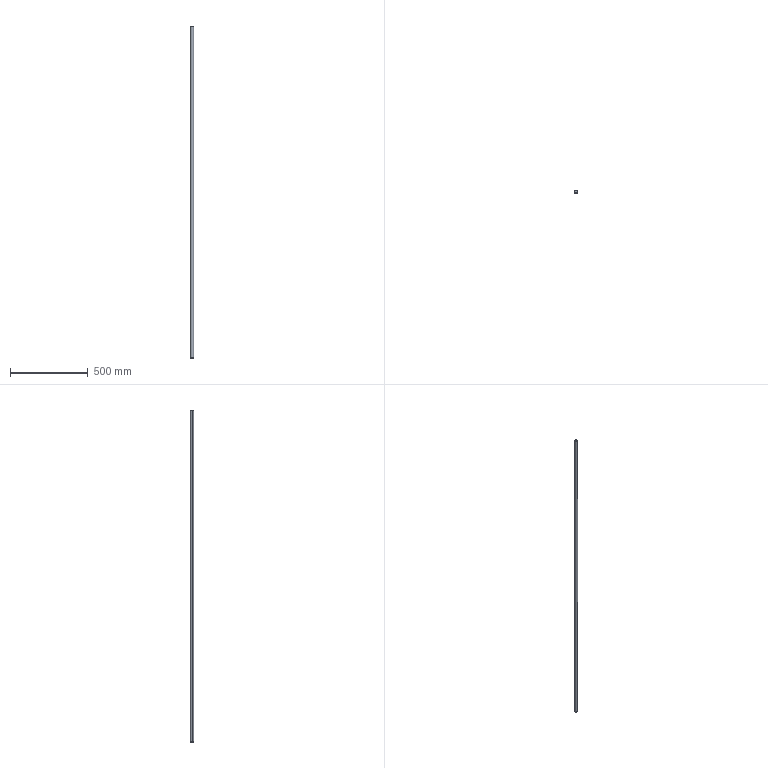Part | SolidWorks | features Chamfer 1, Extrusion 1 | 1 solid | 8 faces | box 20 x 20 x 2135 mm | volume 670495 mm3 | cone 4 | cylinder 2 | plane 2 | commonest cylinder face diameters 20 x2
STEP:
#1=CARTESIAN_POINT('',(8.,0.,2135.));
#2=VERTEX_POINT('',#1);
#3=CARTESIAN_POINT('',(-8.,0.,2135.));
#4=VERTEX_POINT('',#3);
#5=CARTESIAN_POINT('',(0.,0.,2135.));
#6=DIRECTION('',(0.,0.,1.));
#7=DIRECTION('',(1.,0.,0.));
#8=AXIS2_PLACEMENT_3D('',#5,#6,#7);
#9=CIRCLE('',#8,8.);
#10=EDGE_CURVE('',#2,#4,#9,.T.);
#11=ORIENTED_EDGE('',*,*,#10,.F.);
#12=CARTESIAN_POINT('',(10.,0.,2133.));
#13=VERTEX_POINT('',#12);
#14=CARTESIAN_POINT('',(8.,0.,2135.));
#15=DIRECTION('',(0.7071,0.,-0.7071));
#16=VECTOR('',#15,1000.);
#17=LINE('',#14,#16);
#18=EDGE_CURVE('',#2,#13,#17,.T.);
#19=ORIENTED_EDGE('',*,*,#18,.T.);
#20=CARTESIAN_POINT('',(-10.,0.,2133.));
#21=VERTEX_POINT('',#20);
#22=CARTESIAN_POINT('',(0.,0.,2133.));
#23=DIRECTION('',(0.,0.,-1.));
#24=DIRECTION('',(1.,0.,0.));
#25=AXIS2_PLACEMENT_3D('',#22,#23,#24);
#26=CIRCLE('',#25,10.);
#27=EDGE_CURVE('',#21,#13,#26,.T.);
#28=ORIENTED_EDGE('',*,*,#27,.F.);
#29=CARTESIAN_POINT('',(-8.,0.,2135.));
#30=DIRECTION('',(-0.7071,0.,-0.7071));
#31=VECTOR('',#30,1000.);
#32=LINE('',#29,#31);
#33=EDGE_CURVE('',#4,#21,#32,.T.);
#34=ORIENTED_EDGE('',*,*,#33,.F.);
#35=EDGE_LOOP('',(#11,#19,#28,#34));
#36=FACE_OUTER_BOUND('',#35,.T.);
#37=CARTESIAN_POINT('',(0.,0.,2135.));
#38=DIRECTION('',(0.,0.,-1.));
#39=DIRECTION('',(-1.,0.,0.));
#40=AXIS2_PLACEMENT_3D('',#37,#38,#39);
#41=CONICAL_SURFACE('',#40,8.,0.7854);
#42=ADVANCED_FACE('',(#36),#41,.T.);
#43=CARTESIAN_POINT('',(-8.,0.,0.));
#44=VERTEX_POINT('',#43);
#45=CARTESIAN_POINT('',(8.,0.,0.));
#46=VERTEX_POINT('',#45);
#47=CARTESIAN_POINT('',(0.,0.,0.));
#48=DIRECTION('',(0.,0.,-1.));
#49=DIRECTION('',(1.,0.,0.));
#50=AXIS2_PLACEMENT_3D('',#47,#48,#49);
#51=CIRCLE('',#50,8.);
#52=EDGE_CURVE('',#44,#46,#51,.T.);
#53=ORIENTED_EDGE('',*,*,#52,.F.);
#54=CARTESIAN_POINT('',(-10.,0.,2.));
#55=VERTEX_POINT('',#54);
#56=CARTESIAN_POINT('',(-10.,0.,2.));
#57=DIRECTION('',(-0.7071,0.,0.7071));
#58=VECTOR('',#57,1000.);
#59=LINE('',#56,#58);
#60=EDGE_CURVE('',#44,#55,#59,.T.);
#61=ORIENTED_EDGE('',*,*,#60,.T.);
#62=CARTESIAN_POINT('',(10.,0.,2.));
#63=VERTEX_POINT('',#62);
#64=CARTESIAN_POINT('',(0.,0.,2.));
#65=DIRECTION('',(0.,0.,1.));
#66=DIRECTION('',(1.,0.,0.));
#67=AXIS2_PLACEMENT_3D('',#64,#65,#66);
#68=CIRCLE('',#67,10.);
#69=EDGE_CURVE('',#63,#55,#68,.T.);
#70=ORIENTED_EDGE('',*,*,#69,.F.);
#71=CARTESIAN_POINT('',(10.,0.,2.));
#72=DIRECTION('',(0.7071,0.,0.7071));
#73=VECTOR('',#72,1000.);
#74=LINE('',#71,#73);
#75=EDGE_CURVE('',#46,#63,#74,.T.);
#76=ORIENTED_EDGE('',*,*,#75,.F.);
#77=EDGE_LOOP('',(#53,#61,#70,#76));
#78=FACE_OUTER_BOUND('',#77,.T.);
#79=CARTESIAN_POINT('',(0.,0.,2.));
#80=DIRECTION('',(0.,0.,1.));
#81=DIRECTION('',(1.,0.,0.));
#82=AXIS2_PLACEMENT_3D('',#79,#80,#81);
#83=CONICAL_SURFACE('',#82,10.,0.7854);
#84=ADVANCED_FACE('',(#78),#83,.T.);
#85=ORIENTED_EDGE('',*,*,#27,.T.);
#86=CARTESIAN_POINT('',(10.,0.,2135.));
#87=DIRECTION('',(0.,0.,-1.));
#88=VECTOR('',#87,1000.);
#89=LINE('',#86,#88);
#90=EDGE_CURVE('',#13,#63,#89,.T.);
#91=ORIENTED_EDGE('',*,*,#90,.T.);
#92=ORIENTED_EDGE('',*,*,#69,.T.);
#93=CARTESIAN_POINT('',(-10.,0.,2135.));
#94=DIRECTION('',(0.,0.,-1.));
#95=VECTOR('',#94,1000.);
#96=LINE('',#93,#95);
#97=EDGE_CURVE('',#21,#55,#96,.T.);
#98=ORIENTED_EDGE('',*,*,#97,.F.);
#99=EDGE_LOOP('',(#85,#91,#92,#98));
#100=FACE_OUTER_BOUND('',#99,.T.);
#101=CARTESIAN_POINT('',(0.,0.,2135.));
#102=DIRECTION('',(0.,0.,-1.));
#103=DIRECTION('',(-1.,0.,0.));
#104=AXIS2_PLACEMENT_3D('',#101,#102,#103);
#105=CYLINDRICAL_SURFACE('',#104,10.);
#106=ADVANCED_FACE('',(#100),#105,.T.);
#107=ORIENTED_EDGE('',*,*,#90,.F.);
#108=CARTESIAN_POINT('',(0.,0.,2133.));
#109=DIRECTION('',(0.,0.,-1.));
#110=DIRECTION('',(1.,0.,0.));
#111=AXIS2_PLACEMENT_3D('',#108,#109,#110);
#112=CIRCLE('',#111,10.);
#113=EDGE_CURVE('',#13,#21,#112,.T.);
#114=ORIENTED_EDGE('',*,*,#113,.T.);
#115=ORIENTED_EDGE('',*,*,#97,.T.);
#116=CARTESIAN_POINT('',(0.,0.,2.));
#117=DIRECTION('',(0.,0.,1.));
#118=DIRECTION('',(1.,0.,0.));
#119=AXIS2_PLACEMENT_3D('',#116,#117,#118);
#120=CIRCLE('',#119,10.);
#121=EDGE_CURVE('',#55,#63,#120,.T.);
#122=ORIENTED_EDGE('',*,*,#121,.T.);
#123=EDGE_LOOP('',(#107,#114,#115,#122));
#124=FACE_OUTER_BOUND('',#123,.T.);
#125=CARTESIAN_POINT('',(0.,0.,2135.));
#126=DIRECTION('',(0.,0.,-1.));
#127=DIRECTION('',(-1.,0.,0.));
#128=AXIS2_PLACEMENT_3D('',#125,#126,#127);
#129=CYLINDRICAL_SURFACE('',#128,10.);
#130=ADVANCED_FACE('',(#124),#129,.T.);
#131=CARTESIAN_POINT('',(0.,0.,2135.));
#132=DIRECTION('',(0.,0.,1.));
#133=DIRECTION('',(1.,0.,0.));
#134=AXIS2_PLACEMENT_3D('',#131,#132,#133);
#135=CIRCLE('',#134,8.);
#136=EDGE_CURVE('',#4,#2,#135,.T.);
#137=ORIENTED_EDGE('',*,*,#136,.T.);
#138=ORIENTED_EDGE('',*,*,#10,.T.);
#139=EDGE_LOOP('',(#137,#138));
#140=FACE_OUTER_BOUND('',#139,.T.);
#141=CARTESIAN_POINT('',(0.,0.,2135.));
#142=DIRECTION('',(0.,0.,1.));
#143=DIRECTION('',(1.,0.,0.));
#144=AXIS2_PLACEMENT_3D('',#141,#142,#143);
#145=PLANE('',#144);
#146=ADVANCED_FACE('',(#140),#145,.T.);
#147=CARTESIAN_POINT('',(0.,0.,0.));
#148=DIRECTION('',(0.,0.,-1.));
#149=DIRECTION('',(1.,0.,0.));
#150=AXIS2_PLACEMENT_3D('',#147,#148,#149);
#151=CIRCLE('',#150,8.);
#152=EDGE_CURVE('',#46,#44,#151,.T.);
#153=ORIENTED_EDGE('',*,*,#152,.T.);
#154=ORIENTED_EDGE('',*,*,#52,.T.);
#155=EDGE_LOOP('',(#153,#154));
#156=FACE_OUTER_BOUND('',#155,.T.);
#157=CARTESIAN_POINT('',(0.,0.,0.));
#158=DIRECTION('',(0.,0.,1.));
#159=DIRECTION('',(1.,0.,0.));
#160=AXIS2_PLACEMENT_3D('',#157,#158,#159);
#161=PLANE('',#160);
#162=ADVANCED_FACE('',(#156),#161,.F.);
#163=ORIENTED_EDGE('',*,*,#60,.F.);
#164=ORIENTED_EDGE('',*,*,#152,.F.);
#165=ORIENTED_EDGE('',*,*,#75,.T.);
#166=ORIENTED_EDGE('',*,*,#121,.F.);
#167=EDGE_LOOP('',(#163,#164,#165,#166));
#168=FACE_OUTER_BOUND('',#167,.T.);
#169=CARTESIAN_POINT('',(0.,0.,2.));
#170=DIRECTION('',(0.,0.,1.));
#171=DIRECTION('',(1.,0.,0.));
#172=AXIS2_PLACEMENT_3D('',#169,#170,#171);
#173=CONICAL_SURFACE('',#172,10.,0.7854);
#174=ADVANCED_FACE('',(#168),#173,.T.);
#175=ORIENTED_EDGE('',*,*,#18,.F.);
#176=ORIENTED_EDGE('',*,*,#136,.F.);
#177=ORIENTED_EDGE('',*,*,#33,.T.);
#178=ORIENTED_EDGE('',*,*,#113,.F.);
#179=EDGE_LOOP('',(#175,#176,#177,#178));
#180=FACE_OUTER_BOUND('',#179,.T.);
#181=CARTESIAN_POINT('',(0.,0.,2135.));
#182=DIRECTION('',(0.,0.,-1.));
#183=DIRECTION('',(-1.,0.,0.));
#184=AXIS2_PLACEMENT_3D('',#181,#182,#183);
#185=CONICAL_SURFACE('',#184,8.,0.7854);
#186=ADVANCED_FACE('',(#180),#185,.T.);
#187=CLOSED_SHELL('',(#42,#84,#106,#130,#146,#162,#174,#186));
#188=MANIFOLD_SOLID_BREP('',#187);
#189=CARTESIAN_POINT('',(0.,0.,0.));
#190=DIRECTION('',(0.,0.,1.));
#191=DIRECTION('',(1.,0.,0.));
#192=AXIS2_PLACEMENT_3D('',#189,#190,#191);
#193=(LENGTH_UNIT()NAMED_UNIT(*)SI_UNIT(.MILLI.,.METRE.));
#194=UNCERTAINTY_MEASURE_WITH_UNIT(LENGTH_MEASURE(0.00001),#193,'','');
#195=(NAMED_UNIT(*)PLANE_ANGLE_UNIT()SI_UNIT($,.RADIAN.));
#196=(NAMED_UNIT(*)SI_UNIT($,.STERADIAN.)SOLID_ANGLE_UNIT());
#197=(GEOMETRIC_REPRESENTATION_CONTEXT(3)GLOBAL_UNCERTAINTY_ASSIGNED_CONTEXT((#194))GLOBAL_UNIT_ASSIGNED_CONTEXT((#193,#195,#196))REPRESENTATION_CONTEXT('',''));
#198=ADVANCED_BREP_SHAPE_REPRESENTATION('',(#188,#192),#197);